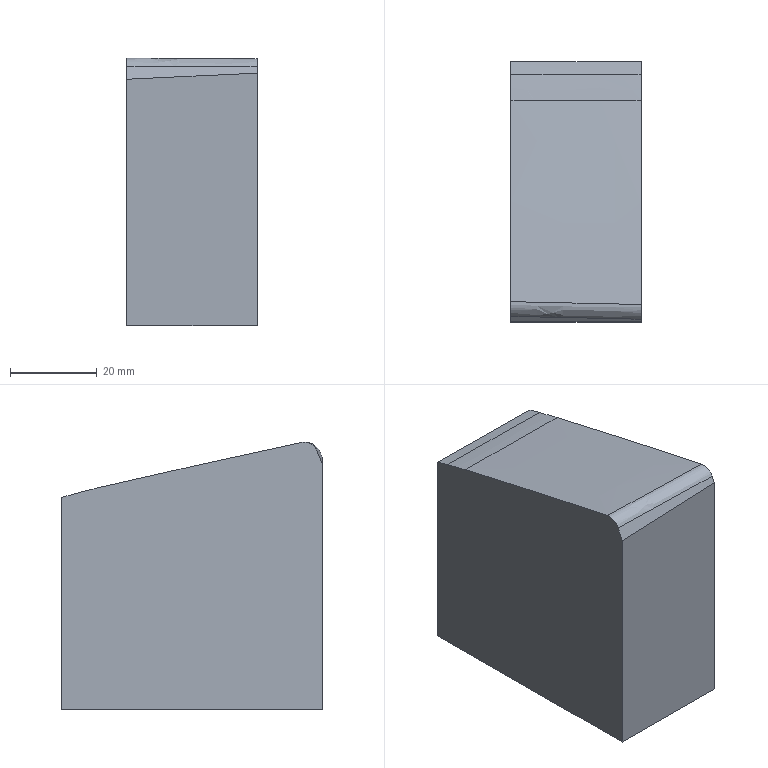Part | NX | features solid 2 | 1 solid | 10 faces | box 30 x 60 x 61.716 mm | volume 100455 mm3 | plane 5 | spline 5
STEP:
#1=CARTESIAN_POINT('',(-145.,690.,-45.));
#2=VERTEX_POINT('',#1);
#3=CARTESIAN_POINT('',(-115.,690.,-45.));
#4=VERTEX_POINT('',#3);
#5=CARTESIAN_POINT('',(-130.,690.,-45.));
#6=DIRECTION('',(1.,0.,0.));
#7=VECTOR('',#6,1000.);
#8=LINE('',#5,#7);
#9=EDGE_CURVE('',#2,#4,#8,.T.);
#10=ORIENTED_EDGE('',*,*,#9,.F.);
#11=CARTESIAN_POINT('',(-145.,750.,-45.));
#12=VERTEX_POINT('',#11);
#13=CARTESIAN_POINT('',(-145.,615.,-45.));
#14=DIRECTION('',(0.,-1.,0.));
#15=VECTOR('',#14,1000.);
#16=LINE('',#13,#15);
#17=EDGE_CURVE('',#2,#12,#16,.F.);
#18=ORIENTED_EDGE('',*,*,#17,.T.);
#19=CARTESIAN_POINT('',(-115.,750.,-45.));
#20=VERTEX_POINT('',#19);
#21=CARTESIAN_POINT('',(-130.,750.,-45.));
#22=DIRECTION('',(-1.,0.,0.));
#23=VECTOR('',#22,1000.);
#24=LINE('',#21,#23);
#25=EDGE_CURVE('',#12,#20,#24,.F.);
#26=ORIENTED_EDGE('',*,*,#25,.T.);
#27=CARTESIAN_POINT('',(-115.,615.,-45.));
#28=DIRECTION('',(0.,-1.,0.));
#29=VECTOR('',#28,1000.);
#30=LINE('',#27,#29);
#31=EDGE_CURVE('',#4,#20,#30,.F.);
#32=ORIENTED_EDGE('',*,*,#31,.F.);
#33=EDGE_LOOP('',(#10,#18,#26,#32));
#34=FACE_BOUND('',#33,.T.);
#35=CARTESIAN_POINT('',(-130.,615.,-45.));
#36=DIRECTION('',(0.,0.,1.));
#37=DIRECTION('',(0.,1.,0.));
#38=AXIS2_PLACEMENT_3D('',#35,#36,#37);
#39=PLANE('',#38);
#40=ADVANCED_FACE('',(#34),#39,.F.);
#41=CARTESIAN_POINT('',(-115.,746.976,4.561));
#42=VERTEX_POINT('',#41);
#43=CARTESIAN_POINT('',(-115.,750.,3.754));
#44=VERTEX_POINT('',#43);
#45=CARTESIAN_POINT('',(-115.,746.976,4.561));
#46=CARTESIAN_POINT('',(-115.,747.984,4.291));
#47=CARTESIAN_POINT('',(-115.,748.992,4.022));
#48=CARTESIAN_POINT('',(-115.,750.,3.754));
#49=B_SPLINE_CURVE_WITH_KNOTS('',3,(#45,#46,#47,#48),.UNSPECIFIED.,.F.,.F.,(4,4),(0.00006785,0.003198),.UNSPECIFIED.);
#50=EDGE_CURVE('',#42,#44,#49,.T.);
#51=ORIENTED_EDGE('',*,*,#50,.F.);
#52=CARTESIAN_POINT('',(-115.,741.156,6.02));
#53=VERTEX_POINT('',#52);
#54=CARTESIAN_POINT('',(-115.,746.976,4.561));
#55=CARTESIAN_POINT('',(-115.,745.044,5.079));
#56=CARTESIAN_POINT('',(-115.,743.105,5.569));
#57=CARTESIAN_POINT('',(-115.,741.156,6.02));
#58=B_SPLINE_CURVE_WITH_KNOTS('',3,(#54,#55,#56,#57),.UNSPECIFIED.,.F.,.F.,(4,4),(0.,0.006),.UNSPECIFIED.);
#59=EDGE_CURVE('',#42,#53,#58,.T.);
#60=ORIENTED_EDGE('',*,*,#59,.T.);
#61=CARTESIAN_POINT('',(-115.,694.002,16.504));
#62=VERTEX_POINT('',#61);
#63=CARTESIAN_POINT('',(-115.,741.156,6.02));
#64=CARTESIAN_POINT('',(-115.,725.469,9.655));
#65=CARTESIAN_POINT('',(-115.,709.751,13.15));
#66=CARTESIAN_POINT('',(-115.,694.001,16.504));
#67=B_SPLINE_CURVE_WITH_KNOTS('',3,(#63,#64,#65,#66),.UNSPECIFIED.,.F.,.F.,(4,4),(0.0003493,0.04866),.UNSPECIFIED.);
#68=EDGE_CURVE('',#53,#62,#67,.T.);
#69=ORIENTED_EDGE('',*,*,#68,.T.);
#70=CARTESIAN_POINT('',(-115.,690.605,14.719));
#71=VERTEX_POINT('',#70);
#72=CARTESIAN_POINT('',(-115.,694.002,16.503));
#73=CARTESIAN_POINT('',(-115.,692.631,16.795));
#74=CARTESIAN_POINT('',(-115.,691.143,16.014));
#75=CARTESIAN_POINT('',(-115.,690.605,14.719));
#76=B_SPLINE_CURVE_WITH_KNOTS('',3,(#72,#73,#74,#75),.UNSPECIFIED.,.F.,.F.,(4,4),(0.,0.004145),.UNSPECIFIED.);
#77=EDGE_CURVE('',#62,#71,#76,.T.);
#78=ORIENTED_EDGE('',*,*,#77,.T.);
#79=CARTESIAN_POINT('',(-115.,690.,13.263));
#80=VERTEX_POINT('',#79);
#81=CARTESIAN_POINT('',(-115.,690.,13.263));
#82=CARTESIAN_POINT('',(-115.,690.202,13.748));
#83=CARTESIAN_POINT('',(-115.,690.403,14.234));
#84=CARTESIAN_POINT('',(-115.,690.605,14.719));
#85=B_SPLINE_CURVE_WITH_KNOTS('',3,(#81,#82,#83,#84),.UNSPECIFIED.,.F.,.F.,(4,4),(0.,0.001577),.UNSPECIFIED.);
#86=EDGE_CURVE('',#80,#71,#85,.T.);
#87=ORIENTED_EDGE('',*,*,#86,.F.);
#88=CARTESIAN_POINT('',(-115.,690.,95.));
#89=DIRECTION('',(0.,0.,1.));
#90=VECTOR('',#89,1000.);
#91=LINE('',#88,#90);
#92=EDGE_CURVE('',#80,#4,#91,.F.);
#93=ORIENTED_EDGE('',*,*,#92,.T.);
#94=ORIENTED_EDGE('',*,*,#31,.T.);
#95=CARTESIAN_POINT('',(-115.,750.,95.));
#96=DIRECTION('',(0.,0.,-1.));
#97=VECTOR('',#96,1000.);
#98=LINE('',#95,#97);
#99=EDGE_CURVE('',#44,#20,#98,.T.);
#100=ORIENTED_EDGE('',*,*,#99,.F.);
#101=EDGE_LOOP('',(#51,#60,#69,#78,#87,#93,#94,#100));
#102=FACE_BOUND('',#101,.T.);
#103=CARTESIAN_POINT('',(-115.,615.,95.));
#104=DIRECTION('',(-1.,0.,0.));
#105=DIRECTION('',(0.,0.,1.));
#106=AXIS2_PLACEMENT_3D('',#103,#104,#105);
#107=PLANE('',#106);
#108=ADVANCED_FACE('',(#102),#107,.F.);
#109=CARTESIAN_POINT('',(-145.,746.938,4.834));
#110=VERTEX_POINT('',#109);
#111=CARTESIAN_POINT('',(-145.,741.128,6.331));
#112=VERTEX_POINT('',#111);
#113=CARTESIAN_POINT('',(-145.,746.938,4.834));
#114=CARTESIAN_POINT('',(-145.,745.013,5.378));
#115=CARTESIAN_POINT('',(-145.,743.077,5.88));
#116=CARTESIAN_POINT('',(-145.,741.128,6.331));
#117=B_SPLINE_CURVE_WITH_KNOTS('',3,(#113,#114,#115,#116),.UNSPECIFIED.,.F.,.F.,(4,4),(0.,0.006001),.UNSPECIFIED.);
#118=EDGE_CURVE('',#110,#112,#117,.T.);
#119=ORIENTED_EDGE('',*,*,#118,.F.);
#120=CARTESIAN_POINT('',(-145.,750.,3.972));
#121=VERTEX_POINT('',#120);
#122=CARTESIAN_POINT('',(-145.,746.938,4.834));
#123=CARTESIAN_POINT('',(-145.,747.958,4.546));
#124=CARTESIAN_POINT('',(-145.,748.979,4.258));
#125=CARTESIAN_POINT('',(-145.,750.,3.972));
#126=B_SPLINE_CURVE_WITH_KNOTS('',3,(#122,#123,#124,#125),.UNSPECIFIED.,.F.,.F.,(4,4),(0.00005297,0.003234),.UNSPECIFIED.);
#127=EDGE_CURVE('',#110,#121,#126,.T.);
#128=ORIENTED_EDGE('',*,*,#127,.T.);
#129=CARTESIAN_POINT('',(-145.,750.,95.));
#130=DIRECTION('',(0.,0.,-1.));
#131=VECTOR('',#130,1000.);
#132=LINE('',#129,#131);
#133=EDGE_CURVE('',#121,#12,#132,.T.);
#134=ORIENTED_EDGE('',*,*,#133,.T.);
#135=ORIENTED_EDGE('',*,*,#17,.F.);
#136=CARTESIAN_POINT('',(-145.,690.,11.857));
#137=VERTEX_POINT('',#136);
#138=CARTESIAN_POINT('',(-145.,690.,95.));
#139=DIRECTION('',(0.,0.,1.));
#140=VECTOR('',#139,1000.);
#141=LINE('',#138,#140);
#142=EDGE_CURVE('',#137,#2,#141,.F.);
#143=ORIENTED_EDGE('',*,*,#142,.F.);
#144=CARTESIAN_POINT('',(-145.,691.251,14.87));
#145=VERTEX_POINT('',#144);
#146=CARTESIAN_POINT('',(-145.,690.,11.857));
#147=CARTESIAN_POINT('',(-145.,690.417,12.862));
#148=CARTESIAN_POINT('',(-145.,690.834,13.866));
#149=CARTESIAN_POINT('',(-145.,691.251,14.87));
#150=B_SPLINE_CURVE_WITH_KNOTS('',3,(#146,#147,#148,#149),.UNSPECIFIED.,.F.,.F.,(4,4),(0.,0.003262),.UNSPECIFIED.);
#151=EDGE_CURVE('',#137,#145,#150,.T.);
#152=ORIENTED_EDGE('',*,*,#151,.T.);
#153=CARTESIAN_POINT('',(-145.,694.647,16.655));
#154=VERTEX_POINT('',#153);
#155=CARTESIAN_POINT('',(-145.,694.647,16.655));
#156=CARTESIAN_POINT('',(-145.,693.276,16.947));
#157=CARTESIAN_POINT('',(-145.,691.788,16.165));
#158=CARTESIAN_POINT('',(-145.,691.251,14.87));
#159=B_SPLINE_CURVE_WITH_KNOTS('',3,(#155,#156,#157,#158),.UNSPECIFIED.,.F.,.F.,(4,4),(0.,0.004145),.UNSPECIFIED.);
#160=EDGE_CURVE('',#154,#145,#159,.T.);
#161=ORIENTED_EDGE('',*,*,#160,.F.);
#162=CARTESIAN_POINT('',(-145.,741.128,6.331));
#163=CARTESIAN_POINT('',(-145.,725.664,9.909));
#164=CARTESIAN_POINT('',(-145.,710.171,13.351));
#165=CARTESIAN_POINT('',(-145.,694.647,16.655));
#166=B_SPLINE_CURVE_WITH_KNOTS('',3,(#162,#163,#164,#165),.UNSPECIFIED.,.F.,.F.,(4,4),(0.0003508,0.04796),.UNSPECIFIED.);
#167=EDGE_CURVE('',#112,#154,#166,.T.);
#168=ORIENTED_EDGE('',*,*,#167,.F.);
#169=EDGE_LOOP('',(#119,#128,#134,#135,#143,#152,#161,#168));
#170=FACE_BOUND('',#169,.T.);
#171=CARTESIAN_POINT('',(-145.,615.,95.));
#172=DIRECTION('',(-1.,0.,0.));
#173=DIRECTION('',(0.,0.,1.));
#174=AXIS2_PLACEMENT_3D('',#171,#172,#173);
#175=PLANE('',#174);
#176=ADVANCED_FACE('',(#170),#175,.T.);
#177=ORIENTED_EDGE('',*,*,#133,.F.);
#178=CARTESIAN_POINT('',(-145.,750.,3.972));
#179=CARTESIAN_POINT('',(-135.,750.,3.912));
#180=CARTESIAN_POINT('',(-125.,750.,3.84));
#181=CARTESIAN_POINT('',(-115.,750.,3.754));
#182=B_SPLINE_CURVE_WITH_KNOTS('',3,(#178,#179,#180,#181),.UNSPECIFIED.,.F.,.F.,(4,4),(0.,0.03),.UNSPECIFIED.);
#183=EDGE_CURVE('',#121,#44,#182,.T.);
#184=ORIENTED_EDGE('',*,*,#183,.T.);
#185=ORIENTED_EDGE('',*,*,#99,.T.);
#186=ORIENTED_EDGE('',*,*,#25,.F.);
#187=EDGE_LOOP('',(#177,#184,#185,#186));
#188=FACE_BOUND('',#187,.T.);
#189=CARTESIAN_POINT('',(-130.,750.,95.));
#190=DIRECTION('',(0.,1.,0.));
#191=DIRECTION('',(0.,0.,-1.));
#192=AXIS2_PLACEMENT_3D('',#189,#190,#191);
#193=PLANE('',#192);
#194=ADVANCED_FACE('',(#188),#193,.T.);
#195=ORIENTED_EDGE('',*,*,#92,.F.);
#196=CARTESIAN_POINT('',(-115.,690.,13.263));
#197=CARTESIAN_POINT('',(-124.997,690.,12.736));
#198=CARTESIAN_POINT('',(-134.997,690.,12.268));
#199=CARTESIAN_POINT('',(-145.,690.,11.857));
#200=B_SPLINE_CURVE_WITH_KNOTS('',3,(#196,#197,#198,#199),.UNSPECIFIED.,.F.,.F.,(4,4),(0.,0.03003),.UNSPECIFIED.);
#201=EDGE_CURVE('',#80,#137,#200,.T.);
#202=ORIENTED_EDGE('',*,*,#201,.T.);
#203=ORIENTED_EDGE('',*,*,#142,.T.);
#204=ORIENTED_EDGE('',*,*,#9,.T.);
#205=EDGE_LOOP('',(#195,#202,#203,#204));
#206=FACE_BOUND('',#205,.T.);
#207=CARTESIAN_POINT('',(-130.,690.,95.));
#208=DIRECTION('',(0.,1.,0.));
#209=DIRECTION('',(0.,0.,-1.));
#210=AXIS2_PLACEMENT_3D('',#207,#208,#209);
#211=PLANE('',#210);
#212=ADVANCED_FACE('',(#206),#211,.F.);
#213=ORIENTED_EDGE('',*,*,#68,.F.);
#214=CARTESIAN_POINT('',(-124.341,741.146,6.124));
#215=VERTEX_POINT('',#214);
#216=CARTESIAN_POINT('',(-124.341,741.146,6.124));
#217=CARTESIAN_POINT('',(-121.369,741.149,6.092));
#218=CARTESIAN_POINT('',(-118.223,741.153,6.057));
#219=CARTESIAN_POINT('',(-115.,741.156,6.02));
#220=B_SPLINE_CURVE_WITH_KNOTS('',3,(#216,#217,#218,#219),.UNSPECIFIED.,.F.,.F.,(4,4),(0.,0.2838),.UNSPECIFIED.);
#221=EDGE_CURVE('',#215,#53,#220,.T.);
#222=ORIENTED_EDGE('',*,*,#221,.F.);
#223=CARTESIAN_POINT('',(-139.566,741.132,6.28));
#224=VERTEX_POINT('',#223);
#225=CARTESIAN_POINT('',(-139.566,741.132,6.28));
#226=CARTESIAN_POINT('',(-134.49,741.137,6.231));
#227=CARTESIAN_POINT('',(-129.418,741.141,6.179));
#228=CARTESIAN_POINT('',(-124.341,741.146,6.124));
#229=B_SPLINE_CURVE_WITH_KNOTS('',3,(#225,#226,#227,#228),.UNSPECIFIED.,.F.,.F.,(4,4),(0.,1.),.UNSPECIFIED.);
#230=EDGE_CURVE('',#224,#215,#229,.T.);
#231=ORIENTED_EDGE('',*,*,#230,.F.);
#232=CARTESIAN_POINT('',(-145.,741.128,6.331));
#233=CARTESIAN_POINT('',(-143.189,741.129,6.314));
#234=CARTESIAN_POINT('',(-141.377,741.13,6.297));
#235=CARTESIAN_POINT('',(-139.566,741.132,6.28));
#236=B_SPLINE_CURVE_WITH_KNOTS('',3,(#232,#233,#234,#235),.UNSPECIFIED.,.F.,.F.,(4,4),(0.8551,1.),.UNSPECIFIED.);
#237=EDGE_CURVE('',#112,#224,#236,.T.);
#238=ORIENTED_EDGE('',*,*,#237,.F.);
#239=ORIENTED_EDGE('',*,*,#167,.T.);
#240=CARTESIAN_POINT('',(-115.,694.001,16.504));
#241=CARTESIAN_POINT('',(-124.999,694.242,16.558));
#242=CARTESIAN_POINT('',(-134.999,694.457,16.608));
#243=CARTESIAN_POINT('',(-145.,694.647,16.655));
#244=B_SPLINE_CURVE_WITH_KNOTS('',3,(#240,#241,#242,#243),.UNSPECIFIED.,.F.,.F.,(4,4),(0.5065,0.9282),.UNSPECIFIED.);
#245=EDGE_CURVE('',#62,#154,#244,.T.);
#246=ORIENTED_EDGE('',*,*,#245,.F.);
#247=EDGE_LOOP('',(#213,#222,#231,#238,#239,#246));
#248=FACE_BOUND('',#247,.T.);
#249=CARTESIAN_POINT('',(-114.82,741.44,5.952));
#250=CARTESIAN_POINT('',(-120.892,741.433,6.022));
#251=CARTESIAN_POINT('',(-126.964,741.428,6.088));
#252=CARTESIAN_POINT('',(-133.036,741.422,6.151));
#253=CARTESIAN_POINT('',(-139.108,741.417,6.211));
#254=CARTESIAN_POINT('',(-145.18,741.412,6.267));
#255=CARTESIAN_POINT('',(-114.82,731.887,8.167));
#256=CARTESIAN_POINT('',(-120.892,731.881,8.236));
#257=CARTESIAN_POINT('',(-126.964,731.876,8.301));
#258=CARTESIAN_POINT('',(-133.036,731.87,8.363));
#259=CARTESIAN_POINT('',(-139.108,731.865,8.422));
#260=CARTESIAN_POINT('',(-145.18,731.86,8.478));
#261=CARTESIAN_POINT('',(-114.82,722.339,10.335));
#262=CARTESIAN_POINT('',(-120.892,722.333,10.403));
#263=CARTESIAN_POINT('',(-126.964,722.327,10.468));
#264=CARTESIAN_POINT('',(-133.036,722.322,10.529));
#265=CARTESIAN_POINT('',(-139.108,722.317,10.588));
#266=CARTESIAN_POINT('',(-145.18,722.312,10.643));
#267=CARTESIAN_POINT('',(-114.82,712.795,12.457));
#268=CARTESIAN_POINT('',(-120.892,712.789,12.524));
#269=CARTESIAN_POINT('',(-126.964,712.783,12.588));
#270=CARTESIAN_POINT('',(-133.036,712.778,12.649));
#271=CARTESIAN_POINT('',(-139.108,712.773,12.706));
#272=CARTESIAN_POINT('',(-145.18,712.768,12.761));
#273=CARTESIAN_POINT('',(-114.82,703.255,14.533));
#274=CARTESIAN_POINT('',(-120.892,703.249,14.599));
#275=CARTESIAN_POINT('',(-126.964,703.243,14.662));
#276=CARTESIAN_POINT('',(-133.036,703.238,14.722));
#277=CARTESIAN_POINT('',(-139.108,703.233,14.779));
#278=CARTESIAN_POINT('',(-145.18,703.228,14.833));
#279=CARTESIAN_POINT('',(-114.82,693.718,16.562));
#280=CARTESIAN_POINT('',(-120.892,693.713,16.628));
#281=CARTESIAN_POINT('',(-126.964,693.707,16.69));
#282=CARTESIAN_POINT('',(-133.036,693.702,16.749));
#283=CARTESIAN_POINT('',(-139.108,693.697,16.806));
#284=CARTESIAN_POINT('',(-145.18,693.692,16.859));
#285=B_SPLINE_SURFACE_WITH_KNOTS('',5,5,((#249,#250,#251,#252,#253,#254),(#255,#256,#257,#258,#259,#260),(#261,#262,#263,#264,#265,#266),(#267,#268,#269,#270,#271,#272),(#273,#274,#275,#276,#277,#278),(#279,#280,#281,#282,#283,#284)),.UNSPECIFIED.,.F.,.F.,.F.,(6,6),(6,6),(0.00278,0.05308),(0.9323,0.96),.PIECEWISE_BEZIER_KNOTS.);
#286=ADVANCED_FACE('',(#248),#285,.F.);
#287=ORIENTED_EDGE('',*,*,#77,.F.);
#288=ORIENTED_EDGE('',*,*,#245,.T.);
#289=ORIENTED_EDGE('',*,*,#160,.T.);
#290=CARTESIAN_POINT('',(-134.081,691.034,14.818));
#291=VERTEX_POINT('',#290);
#292=CARTESIAN_POINT('',(-134.081,691.034,14.818));
#293=CARTESIAN_POINT('',(-137.721,691.109,14.836));
#294=CARTESIAN_POINT('',(-141.36,691.182,14.853));
#295=CARTESIAN_POINT('',(-145.,691.251,14.87));
#296=B_SPLINE_CURVE_WITH_KNOTS('',3,(#292,#293,#294,#295),.UNSPECIFIED.,.F.,.F.,(4,4),(0.,0.6096),.UNSPECIFIED.);
#297=EDGE_CURVE('',#291,#145,#296,.T.);
#298=ORIENTED_EDGE('',*,*,#297,.F.);
#299=CARTESIAN_POINT('',(-115.,690.605,14.719));
#300=CARTESIAN_POINT('',(-121.36,690.758,14.754));
#301=CARTESIAN_POINT('',(-127.721,690.901,14.787));
#302=CARTESIAN_POINT('',(-134.081,691.034,14.818));
#303=B_SPLINE_CURVE_WITH_KNOTS('',3,(#299,#300,#301,#302),.UNSPECIFIED.,.F.,.F.,(4,4),(0.6427,1.),.UNSPECIFIED.);
#304=EDGE_CURVE('',#71,#291,#303,.T.);
#305=ORIENTED_EDGE('',*,*,#304,.F.);
#306=EDGE_LOOP('',(#287,#288,#289,#298,#305));
#307=FACE_BOUND('',#306,.T.);
#308=CARTESIAN_POINT('',(-114.82,690.601,14.718));
#309=CARTESIAN_POINT('',(-114.808,690.92,15.487));
#310=CARTESIAN_POINT('',(-114.79,691.505,16.145));
#311=CARTESIAN_POINT('',(-114.768,692.308,16.567));
#312=CARTESIAN_POINT('',(-114.746,693.181,16.675));
#313=CARTESIAN_POINT('',(-114.728,693.995,16.502));
#314=CARTESIAN_POINT('',(-120.906,690.748,14.752));
#315=CARTESIAN_POINT('',(-120.894,691.067,15.52));
#316=CARTESIAN_POINT('',(-120.877,691.652,16.178));
#317=CARTESIAN_POINT('',(-120.856,692.455,16.6));
#318=CARTESIAN_POINT('',(-120.836,693.329,16.709));
#319=CARTESIAN_POINT('',(-120.818,694.142,16.535));
#320=CARTESIAN_POINT('',(-126.992,690.887,14.783));
#321=CARTESIAN_POINT('',(-126.981,691.206,15.552));
#322=CARTESIAN_POINT('',(-126.965,691.791,16.21));
#323=CARTESIAN_POINT('',(-126.945,692.594,16.632));
#324=CARTESIAN_POINT('',(-126.925,693.467,16.741));
#325=CARTESIAN_POINT('',(-126.908,694.281,16.567));
#326=CARTESIAN_POINT('',(-133.079,691.017,14.814));
#327=CARTESIAN_POINT('',(-133.068,691.336,15.583));
#328=CARTESIAN_POINT('',(-133.053,691.922,16.241));
#329=CARTESIAN_POINT('',(-133.034,692.724,16.662));
#330=CARTESIAN_POINT('',(-133.015,693.598,16.771));
#331=CARTESIAN_POINT('',(-132.999,694.412,16.598));
#332=CARTESIAN_POINT('',(-139.166,691.14,14.843));
#333=CARTESIAN_POINT('',(-139.156,691.459,15.612));
#334=CARTESIAN_POINT('',(-139.141,692.045,16.27));
#335=CARTESIAN_POINT('',(-139.123,692.847,16.692));
#336=CARTESIAN_POINT('',(-139.105,693.721,16.801));
#337=CARTESIAN_POINT('',(-139.09,694.535,16.627));
#338=CARTESIAN_POINT('',(-145.253,691.255,14.871));
#339=CARTESIAN_POINT('',(-145.243,691.574,15.64));
#340=CARTESIAN_POINT('',(-145.229,692.16,16.298));
#341=CARTESIAN_POINT('',(-145.212,692.962,16.72));
#342=CARTESIAN_POINT('',(-145.195,693.836,16.829));
#343=CARTESIAN_POINT('',(-145.181,694.65,16.656));
#344=B_SPLINE_SURFACE_WITH_KNOTS('',5,5,((#308,#309,#310,#311,#312,#313),(#314,#315,#316,#317,#318,#319),(#320,#321,#322,#323,#324,#325),(#326,#327,#328,#329,#330,#331),(#332,#333,#334,#335,#336,#337),(#338,#339,#340,#341,#342,#343)),.UNSPECIFIED.,.F.,.F.,.F.,(6,6),(6,6),(0.3249,0.6016),(0.,1.),.PIECEWISE_BEZIER_KNOTS.);
#345=ADVANCED_FACE('',(#307),#344,.F.);
#346=ORIENTED_EDGE('',*,*,#59,.F.);
#347=CARTESIAN_POINT('',(-125.136,746.963,4.661));
#348=VERTEX_POINT('',#347);
#349=CARTESIAN_POINT('',(-125.136,746.963,4.661));
#350=CARTESIAN_POINT('',(-121.757,746.967,4.629));
#351=CARTESIAN_POINT('',(-118.379,746.971,4.596));
#352=CARTESIAN_POINT('',(-115.,746.976,4.561));
#353=B_SPLINE_CURVE_WITH_KNOTS('',3,(#349,#350,#351,#352),.UNSPECIFIED.,.F.,.F.,(4,4),(0.,0.2034),.UNSPECIFIED.);
#354=EDGE_CURVE('',#348,#42,#353,.T.);
#355=ORIENTED_EDGE('',*,*,#354,.F.);
#356=CARTESIAN_POINT('',(-145.,746.938,4.834));
#357=CARTESIAN_POINT('',(-138.379,746.946,4.781));
#358=CARTESIAN_POINT('',(-131.757,746.954,4.724));
#359=CARTESIAN_POINT('',(-125.136,746.963,4.661));
#360=B_SPLINE_CURVE_WITH_KNOTS('',3,(#356,#357,#358,#359),.UNSPECIFIED.,.F.,.F.,(4,4),(0.2944,1.),.UNSPECIFIED.);
#361=EDGE_CURVE('',#110,#348,#360,.T.);
#362=ORIENTED_EDGE('',*,*,#361,.F.);
#363=ORIENTED_EDGE('',*,*,#118,.T.);
#364=ORIENTED_EDGE('',*,*,#237,.T.);
#365=ORIENTED_EDGE('',*,*,#230,.T.);
#366=ORIENTED_EDGE('',*,*,#221,.T.);
#367=EDGE_LOOP('',(#346,#355,#362,#363,#364,#365,#366));
#368=FACE_BOUND('',#367,.T.);
#369=CARTESIAN_POINT('',(-148.185,746.934,4.859));
#370=CARTESIAN_POINT('',(-147.427,745.781,5.182));
#371=CARTESIAN_POINT('',(-146.67,744.627,5.504));
#372=CARTESIAN_POINT('',(-146.089,743.465,5.8));
#373=CARTESIAN_POINT('',(-145.647,742.296,6.067));
#374=CARTESIAN_POINT('',(-145.207,741.127,6.333));
#375=CARTESIAN_POINT('',(-143.416,746.94,4.822));
#376=CARTESIAN_POINT('',(-142.618,745.786,5.141));
#377=CARTESIAN_POINT('',(-141.82,744.631,5.461));
#378=CARTESIAN_POINT('',(-141.192,743.469,5.754));
#379=CARTESIAN_POINT('',(-140.701,742.301,6.021));
#380=CARTESIAN_POINT('',(-140.211,741.132,6.287));
#381=CARTESIAN_POINT('',(-138.647,746.945,4.783));
#382=CARTESIAN_POINT('',(-137.808,745.791,5.099));
#383=CARTESIAN_POINT('',(-136.97,744.636,5.415));
#384=CARTESIAN_POINT('',(-136.296,743.473,5.707));
#385=CARTESIAN_POINT('',(-135.754,742.305,5.973));
#386=CARTESIAN_POINT('',(-135.214,741.136,6.238));
#387=CARTESIAN_POINT('',(-133.878,746.951,4.743));
#388=CARTESIAN_POINT('',(-132.999,745.796,5.055));
#389=CARTESIAN_POINT('',(-132.12,744.64,5.368));
#390=CARTESIAN_POINT('',(-131.4,743.478,5.658));
#391=CARTESIAN_POINT('',(-130.807,742.309,5.923));
#392=CARTESIAN_POINT('',(-130.217,741.141,6.188));
#393=CARTESIAN_POINT('',(-129.109,746.957,4.7));
#394=CARTESIAN_POINT('',(-128.189,745.801,5.009));
#395=CARTESIAN_POINT('',(-127.27,744.645,5.319));
#396=CARTESIAN_POINT('',(-126.503,743.482,5.607));
#397=CARTESIAN_POINT('',(-125.861,742.314,5.871));
#398=CARTESIAN_POINT('',(-125.22,741.145,6.135));
#399=CARTESIAN_POINT('',(-124.34,746.963,4.655));
#400=CARTESIAN_POINT('',(-123.38,745.807,4.961));
#401=CARTESIAN_POINT('',(-122.42,744.65,5.268));
#402=CARTESIAN_POINT('',(-121.607,743.487,5.554));
#403=CARTESIAN_POINT('',(-120.914,742.319,5.818));
#404=CARTESIAN_POINT('',(-120.223,741.15,6.081));
#405=CARTESIAN_POINT('',(-119.571,746.97,4.608));
#406=CARTESIAN_POINT('',(-118.57,745.813,4.911));
#407=CARTESIAN_POINT('',(-117.57,744.655,5.214));
#408=CARTESIAN_POINT('',(-116.711,743.492,5.498));
#409=CARTESIAN_POINT('',(-115.967,742.324,5.761));
#410=CARTESIAN_POINT('',(-115.227,741.156,6.024));
#411=CARTESIAN_POINT('',(-114.802,746.976,4.559));
#412=CARTESIAN_POINT('',(-113.761,745.819,4.859));
#413=CARTESIAN_POINT('',(-112.72,744.661,5.159));
#414=CARTESIAN_POINT('',(-111.814,743.498,5.441));
#415=CARTESIAN_POINT('',(-111.021,742.33,5.703));
#416=CARTESIAN_POINT('',(-110.23,741.161,5.965));
#417=B_SPLINE_SURFACE_WITH_KNOTS('',7,5,((#369,#370,#371,#372,#373,#374),(#375,#376,#377,#378,#379,#380),(#381,#382,#383,#384,#385,#386),(#387,#388,#389,#390,#391,#392),(#393,#394,#395,#396,#397,#398),(#399,#400,#401,#402,#403,#404),(#405,#406,#407,#408,#409,#410),(#411,#412,#413,#414,#415,#416)),.UNSPECIFIED.,.F.,.F.,.F.,(8,8),(6,6),(0.2322,0.4174),(0.,1.),.PIECEWISE_BEZIER_KNOTS.);
#418=ADVANCED_FACE('',(#368),#417,.F.);
#419=ORIENTED_EDGE('',*,*,#354,.T.);
#420=ORIENTED_EDGE('',*,*,#50,.T.);
#421=ORIENTED_EDGE('',*,*,#183,.F.);
#422=ORIENTED_EDGE('',*,*,#127,.F.);
#423=ORIENTED_EDGE('',*,*,#361,.T.);
#424=EDGE_LOOP('',(#419,#420,#421,#422,#423));
#425=FACE_BOUND('',#424,.T.);
#426=CARTESIAN_POINT('',(-145.184,746.919,4.841));
#427=CARTESIAN_POINT('',(-147.271,750.017,3.981));
#428=CARTESIAN_POINT('',(-140.445,746.923,4.804));
#429=CARTESIAN_POINT('',(-142.639,750.02,3.953));
#430=CARTESIAN_POINT('',(-135.706,746.926,4.765));
#431=CARTESIAN_POINT('',(-138.006,750.022,3.923));
#432=CARTESIAN_POINT('',(-130.967,746.93,4.724));
#433=CARTESIAN_POINT('',(-133.373,750.025,3.892));
#434=CARTESIAN_POINT('',(-126.228,746.933,4.681));
#435=CARTESIAN_POINT('',(-128.741,750.028,3.858));
#436=CARTESIAN_POINT('',(-121.49,746.937,4.636));
#437=CARTESIAN_POINT('',(-124.108,750.031,3.822));
#438=CARTESIAN_POINT('',(-116.752,746.941,4.588));
#439=CARTESIAN_POINT('',(-119.475,750.034,3.783));
#440=CARTESIAN_POINT('',(-112.014,746.946,4.539));
#441=CARTESIAN_POINT('',(-114.842,750.038,3.743));
#442=B_SPLINE_SURFACE_WITH_KNOTS('',7,1,((#426,#427),(#428,#429),(#430,#431),(#432,#433),(#434,#435),(#436,#437),(#438,#439),(#440,#441)),.RULED_SURF.,.F.,.F.,.F.,(8,8),(2,2),(0.2488,0.4327),(0.2581,0.537),.PIECEWISE_BEZIER_KNOTS.);
#443=ADVANCED_FACE('',(#425),#442,.T.);
#444=ORIENTED_EDGE('',*,*,#201,.F.);
#445=ORIENTED_EDGE('',*,*,#86,.T.);
#446=ORIENTED_EDGE('',*,*,#304,.T.);
#447=ORIENTED_EDGE('',*,*,#297,.T.);
#448=ORIENTED_EDGE('',*,*,#151,.F.);
#449=EDGE_LOOP('',(#444,#445,#446,#447,#448));
#450=FACE_BOUND('',#449,.T.);
#451=CARTESIAN_POINT('',(-114.91,689.343,11.685));
#452=CARTESIAN_POINT('',(-120.998,689.49,11.719));
#453=CARTESIAN_POINT('',(-127.087,689.629,11.751));
#454=CARTESIAN_POINT('',(-133.176,689.76,11.782));
#455=CARTESIAN_POINT('',(-139.265,689.884,11.812));
#456=CARTESIAN_POINT('',(-145.354,689.999,11.841));
#457=CARTESIAN_POINT('',(-114.735,690.606,14.736));
#458=CARTESIAN_POINT('',(-120.824,690.753,14.77));
#459=CARTESIAN_POINT('',(-126.912,690.893,14.802));
#460=CARTESIAN_POINT('',(-133.001,691.024,14.833));
#461=CARTESIAN_POINT('',(-139.09,691.147,14.863));
#462=CARTESIAN_POINT('',(-145.179,691.263,14.892));
#463=B_SPLINE_SURFACE_WITH_KNOTS('',1,5,((#451,#452,#453,#454,#455,#456),(#457,#458,#459,#460,#461,#462)),.SURF_OF_LINEAR_EXTRUSION.,.F.,.F.,.F.,(2,2),(6,6),(0.6182,0.8387),(0.2128,0.3945),.PIECEWISE_BEZIER_KNOTS.);
#464=ADVANCED_FACE('',(#450),#463,.T.);
#465=CLOSED_SHELL('',(#40,#108,#176,#194,#212,#286,#345,#418,#443,#464));
#466=MANIFOLD_SOLID_BREP('',#465);
#467=(LENGTH_UNIT()NAMED_UNIT(*)SI_UNIT(.MILLI.,.METRE.));
#468=UNCERTAINTY_MEASURE_WITH_UNIT(LENGTH_MEASURE(0.1078),#467,'','');
#469=(NAMED_UNIT(*)PLANE_ANGLE_UNIT()SI_UNIT($,.RADIAN.));
#470=(NAMED_UNIT(*)SI_UNIT($,.STERADIAN.)SOLID_ANGLE_UNIT());
#471=(GEOMETRIC_REPRESENTATION_CONTEXT(3)GLOBAL_UNCERTAINTY_ASSIGNED_CONTEXT((#468))GLOBAL_UNIT_ASSIGNED_CONTEXT((#467,#469,#470))REPRESENTATION_CONTEXT('',''));
#472=ADVANCED_BREP_SHAPE_REPRESENTATION('',(#466),#471);